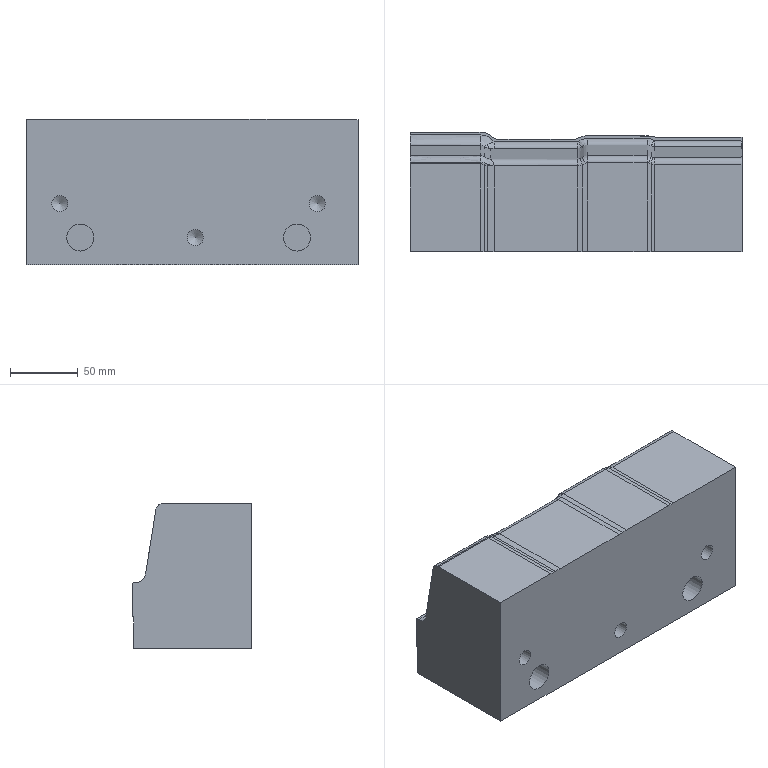Part | NX | features solid 2 | 1 solid | 73 faces | box 245 x 88.207 x 107.259 mm | volume 2041694 mm3 | spline 38 | plane 17 | cylinder 15 | cone 3 | commonest cylinder face diameters 10 x6 12 x5 14 x2 20 x2